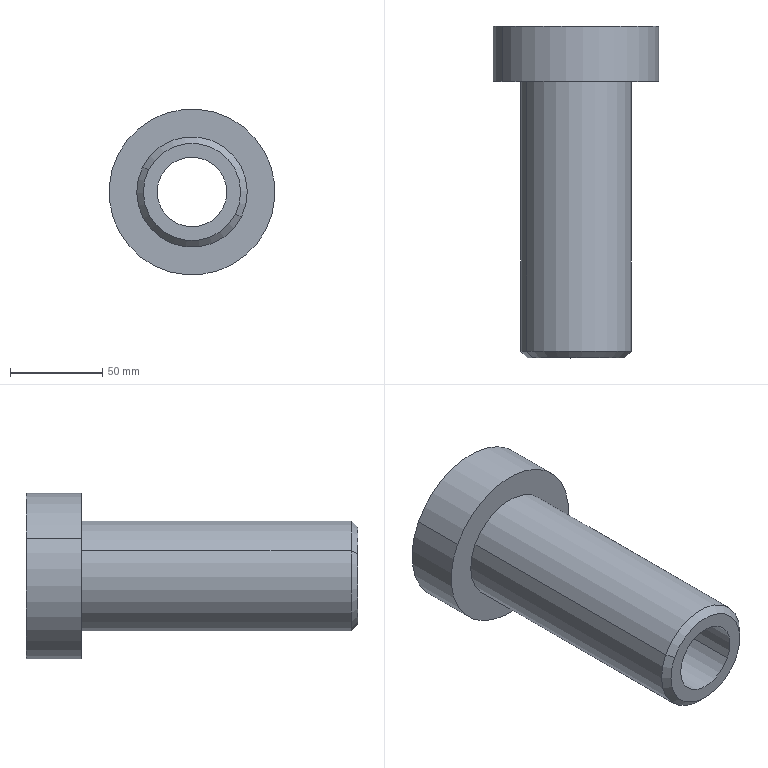Part | STEP file | Scale factor 1[11] | 1 solid | 11 faces | box 90 x 180 x 90 mm | volume 411797 mm3 | cylinder 6 | plane 3 | cone 2 | commonest cylinder face diameters 37.8 x2 60 x2 90 x2
STEP:
#1=CARTESIAN_POINT('',(-772.257,-401.273,3250.492));
#2=VERTEX_POINT('',#1);
#3=CARTESIAN_POINT('',(-725.219,-401.273,3226.508));
#4=VERTEX_POINT('',#3);
#5=CARTESIAN_POINT('',(-748.738,-401.273,3238.5));
#6=DIRECTION('',(0.,-1.,0.));
#7=DIRECTION('',(-0.8909,0.,0.4543));
#8=AXIS2_PLACEMENT_3D('',#5,#6,#7);
#9=CIRCLE('',#8,26.4);
#10=EDGE_CURVE('',#2,#4,#9,.T.);
#11=ORIENTED_EDGE('',*,*,#10,.F.);
#12=CARTESIAN_POINT('',(-775.464,-397.673,3252.128));
#13=VERTEX_POINT('',#12);
#14=CARTESIAN_POINT('',(-772.257,-401.273,3250.492));
#15=DIRECTION('',(-0.6299,0.7071,0.3212));
#16=VECTOR('',#15,1000.);
#17=LINE('',#14,#16);
#18=EDGE_CURVE('',#2,#13,#17,.T.);
#19=ORIENTED_EDGE('',*,*,#18,.T.);
#20=CARTESIAN_POINT('',(-722.012,-397.673,3224.872));
#21=VERTEX_POINT('',#20);
#22=CARTESIAN_POINT('',(-748.738,-397.673,3238.5));
#23=DIRECTION('',(0.,1.,0.));
#24=DIRECTION('',(-0.8909,0.,0.4543));
#25=AXIS2_PLACEMENT_3D('',#22,#23,#24);
#26=CIRCLE('',#25,30.);
#27=EDGE_CURVE('',#21,#13,#26,.T.);
#28=ORIENTED_EDGE('',*,*,#27,.F.);
#29=CARTESIAN_POINT('',(-725.219,-401.273,3226.508));
#30=DIRECTION('',(0.6299,0.7071,-0.3212));
#31=VECTOR('',#30,1000.);
#32=LINE('',#29,#31);
#33=EDGE_CURVE('',#4,#21,#32,.T.);
#34=ORIENTED_EDGE('',*,*,#33,.F.);
#35=EDGE_LOOP('',(#11,#19,#28,#34));
#36=FACE_OUTER_BOUND('',#35,.T.);
#37=CARTESIAN_POINT('',(-748.738,-401.273,3238.5));
#38=DIRECTION('',(0.,1.,0.));
#39=DIRECTION('',(-0.8909,0.,0.4543));
#40=AXIS2_PLACEMENT_3D('',#37,#38,#39);
#41=CONICAL_SURFACE('',#40,26.4,0.7854);
#42=ADVANCED_FACE('',(#36),#41,.T.);
#43=CARTESIAN_POINT('',(-731.901,-401.273,3229.915));
#44=VERTEX_POINT('',#43);
#45=CARTESIAN_POINT('',(-765.576,-401.273,3247.085));
#46=VERTEX_POINT('',#45);
#47=CARTESIAN_POINT('',(-748.738,-401.273,3238.5));
#48=DIRECTION('',(0.,-1.,0.));
#49=DIRECTION('',(-0.8909,0.,0.4543));
#50=AXIS2_PLACEMENT_3D('',#47,#48,#49);
#51=CIRCLE('',#50,18.9);
#52=EDGE_CURVE('',#44,#46,#51,.T.);
#53=ORIENTED_EDGE('',*,*,#52,.T.);
#54=CARTESIAN_POINT('',(-765.576,-221.273,3247.085));
#55=VERTEX_POINT('',#54);
#56=CARTESIAN_POINT('',(-765.576,-431.273,3247.085));
#57=DIRECTION('',(0.,1.,0.));
#58=VECTOR('',#57,1000.);
#59=LINE('',#56,#58);
#60=EDGE_CURVE('',#46,#55,#59,.T.);
#61=ORIENTED_EDGE('',*,*,#60,.T.);
#62=CARTESIAN_POINT('',(-731.901,-221.273,3229.915));
#63=VERTEX_POINT('',#62);
#64=CARTESIAN_POINT('',(-748.738,-221.273,3238.5));
#65=DIRECTION('',(0.,1.,0.));
#66=DIRECTION('',(0.8909,0.,-0.4543));
#67=AXIS2_PLACEMENT_3D('',#64,#65,#66);
#68=CIRCLE('',#67,18.9);
#69=EDGE_CURVE('',#55,#63,#68,.T.);
#70=ORIENTED_EDGE('',*,*,#69,.T.);
#71=CARTESIAN_POINT('',(-731.901,-431.273,3229.915));
#72=DIRECTION('',(0.,1.,0.));
#73=VECTOR('',#72,1000.);
#74=LINE('',#71,#73);
#75=EDGE_CURVE('',#44,#63,#74,.T.);
#76=ORIENTED_EDGE('',*,*,#75,.F.);
#77=EDGE_LOOP('',(#53,#61,#70,#76));
#78=FACE_OUTER_BOUND('',#77,.T.);
#79=CARTESIAN_POINT('',(-748.738,-431.273,3238.5));
#80=DIRECTION('',(0.,1.,0.));
#81=DIRECTION('',(-0.8909,0.,0.4543));
#82=AXIS2_PLACEMENT_3D('',#79,#80,#81);
#83=CYLINDRICAL_SURFACE('',#82,18.9);
#84=ADVANCED_FACE('',(#78),#83,.F.);
#85=ORIENTED_EDGE('',*,*,#27,.T.);
#86=CARTESIAN_POINT('',(-775.464,-251.273,3252.128));
#87=VERTEX_POINT('',#86);
#88=CARTESIAN_POINT('',(-775.464,-401.273,3252.128));
#89=DIRECTION('',(0.,1.,0.));
#90=VECTOR('',#89,1000.);
#91=LINE('',#88,#90);
#92=EDGE_CURVE('',#13,#87,#91,.T.);
#93=ORIENTED_EDGE('',*,*,#92,.T.);
#94=CARTESIAN_POINT('',(-722.012,-251.273,3224.872));
#95=VERTEX_POINT('',#94);
#96=CARTESIAN_POINT('',(-748.738,-251.273,3238.5));
#97=DIRECTION('',(0.,-1.,0.));
#98=DIRECTION('',(-0.8909,0.,0.4543));
#99=AXIS2_PLACEMENT_3D('',#96,#97,#98);
#100=CIRCLE('',#99,30.);
#101=EDGE_CURVE('',#87,#95,#100,.T.);
#102=ORIENTED_EDGE('',*,*,#101,.T.);
#103=CARTESIAN_POINT('',(-722.012,-401.273,3224.872));
#104=DIRECTION('',(0.,1.,0.));
#105=VECTOR('',#104,1000.);
#106=LINE('',#103,#105);
#107=EDGE_CURVE('',#21,#95,#106,.T.);
#108=ORIENTED_EDGE('',*,*,#107,.F.);
#109=EDGE_LOOP('',(#85,#93,#102,#108));
#110=FACE_OUTER_BOUND('',#109,.T.);
#111=CARTESIAN_POINT('',(-748.738,-401.273,3238.5));
#112=DIRECTION('',(0.,1.,0.));
#113=DIRECTION('',(-0.8909,0.,0.4543));
#114=AXIS2_PLACEMENT_3D('',#111,#112,#113);
#115=CYLINDRICAL_SURFACE('',#114,30.);
#116=ADVANCED_FACE('',(#110),#115,.T.);
#117=CARTESIAN_POINT('',(-788.827,-251.273,3258.942));
#118=VERTEX_POINT('',#117);
#119=CARTESIAN_POINT('',(-708.649,-251.273,3218.058));
#120=VERTEX_POINT('',#119);
#121=CARTESIAN_POINT('',(-748.738,-251.273,3238.5));
#122=DIRECTION('',(0.,-1.,0.));
#123=DIRECTION('',(-0.8909,0.,0.4543));
#124=AXIS2_PLACEMENT_3D('',#121,#122,#123);
#125=CIRCLE('',#124,45.);
#126=EDGE_CURVE('',#118,#120,#125,.T.);
#127=ORIENTED_EDGE('',*,*,#126,.F.);
#128=CARTESIAN_POINT('',(-788.827,-221.273,3258.942));
#129=VERTEX_POINT('',#128);
#130=CARTESIAN_POINT('',(-788.827,-251.273,3258.942));
#131=DIRECTION('',(0.,1.,0.));
#132=VECTOR('',#131,1000.);
#133=LINE('',#130,#132);
#134=EDGE_CURVE('',#118,#129,#133,.T.);
#135=ORIENTED_EDGE('',*,*,#134,.T.);
#136=CARTESIAN_POINT('',(-708.649,-221.273,3218.058));
#137=VERTEX_POINT('',#136);
#138=CARTESIAN_POINT('',(-748.738,-221.273,3238.5));
#139=DIRECTION('',(0.,-1.,0.));
#140=DIRECTION('',(-0.8909,0.,0.4543));
#141=AXIS2_PLACEMENT_3D('',#138,#139,#140);
#142=CIRCLE('',#141,45.);
#143=EDGE_CURVE('',#129,#137,#142,.T.);
#144=ORIENTED_EDGE('',*,*,#143,.T.);
#145=CARTESIAN_POINT('',(-708.649,-251.273,3218.058));
#146=DIRECTION('',(0.,1.,0.));
#147=VECTOR('',#146,1000.);
#148=LINE('',#145,#147);
#149=EDGE_CURVE('',#120,#137,#148,.T.);
#150=ORIENTED_EDGE('',*,*,#149,.F.);
#151=EDGE_LOOP('',(#127,#135,#144,#150));
#152=FACE_OUTER_BOUND('',#151,.T.);
#153=CARTESIAN_POINT('',(-748.738,-251.273,3238.5));
#154=DIRECTION('',(0.,1.,0.));
#155=DIRECTION('',(-0.8909,0.,0.4543));
#156=AXIS2_PLACEMENT_3D('',#153,#154,#155);
#157=CYLINDRICAL_SURFACE('',#156,45.);
#158=ADVANCED_FACE('',(#152),#157,.T.);
#159=ORIENTED_EDGE('',*,*,#134,.F.);
#160=CARTESIAN_POINT('',(-748.738,-251.273,3238.5));
#161=DIRECTION('',(0.,-1.,0.));
#162=DIRECTION('',(-0.8909,0.,0.4543));
#163=AXIS2_PLACEMENT_3D('',#160,#161,#162);
#164=CIRCLE('',#163,45.);
#165=EDGE_CURVE('',#120,#118,#164,.T.);
#166=ORIENTED_EDGE('',*,*,#165,.F.);
#167=ORIENTED_EDGE('',*,*,#149,.T.);
#168=CARTESIAN_POINT('',(-748.738,-221.273,3238.5));
#169=DIRECTION('',(0.,-1.,0.));
#170=DIRECTION('',(-0.8909,0.,0.4543));
#171=AXIS2_PLACEMENT_3D('',#168,#169,#170);
#172=CIRCLE('',#171,45.);
#173=EDGE_CURVE('',#137,#129,#172,.T.);
#174=ORIENTED_EDGE('',*,*,#173,.T.);
#175=EDGE_LOOP('',(#159,#166,#167,#174));
#176=FACE_OUTER_BOUND('',#175,.T.);
#177=CARTESIAN_POINT('',(-748.738,-251.273,3238.5));
#178=DIRECTION('',(0.,1.,0.));
#179=DIRECTION('',(-0.8909,0.,0.4543));
#180=AXIS2_PLACEMENT_3D('',#177,#178,#179);
#181=CYLINDRICAL_SURFACE('',#180,45.);
#182=ADVANCED_FACE('',(#176),#181,.T.);
#183=CARTESIAN_POINT('',(-748.738,-251.273,3238.5));
#184=DIRECTION('',(0.,-1.,0.));
#185=DIRECTION('',(-0.8909,0.,0.4543));
#186=AXIS2_PLACEMENT_3D('',#183,#184,#185);
#187=CIRCLE('',#186,30.);
#188=EDGE_CURVE('',#95,#87,#187,.T.);
#189=ORIENTED_EDGE('',*,*,#188,.F.);
#190=ORIENTED_EDGE('',*,*,#101,.F.);
#191=EDGE_LOOP('',(#189,#190));
#192=FACE_BOUND('',#191,.T.);
#193=ORIENTED_EDGE('',*,*,#165,.T.);
#194=ORIENTED_EDGE('',*,*,#126,.T.);
#195=EDGE_LOOP('',(#193,#194));
#196=FACE_OUTER_BOUND('',#195,.T.);
#197=CARTESIAN_POINT('',(-748.738,-251.273,3238.5));
#198=DIRECTION('',(0.,-1.,0.));
#199=DIRECTION('',(0.8909,0.,-0.4543));
#200=AXIS2_PLACEMENT_3D('',#197,#198,#199);
#201=PLANE('',#200);
#202=ADVANCED_FACE('',(#192,#196),#201,.T.);
#203=CARTESIAN_POINT('',(-748.738,-221.273,3238.5));
#204=DIRECTION('',(0.,1.,0.));
#205=DIRECTION('',(0.8909,0.,-0.4543));
#206=AXIS2_PLACEMENT_3D('',#203,#204,#205);
#207=CIRCLE('',#206,18.9);
#208=EDGE_CURVE('',#63,#55,#207,.T.);
#209=ORIENTED_EDGE('',*,*,#208,.F.);
#210=ORIENTED_EDGE('',*,*,#69,.F.);
#211=EDGE_LOOP('',(#209,#210));
#212=FACE_BOUND('',#211,.T.);
#213=ORIENTED_EDGE('',*,*,#173,.F.);
#214=ORIENTED_EDGE('',*,*,#143,.F.);
#215=EDGE_LOOP('',(#213,#214));
#216=FACE_OUTER_BOUND('',#215,.T.);
#217=CARTESIAN_POINT('',(-748.738,-221.273,3238.5));
#218=DIRECTION('',(0.,-1.,0.));
#219=DIRECTION('',(0.8909,0.,-0.4543));
#220=AXIS2_PLACEMENT_3D('',#217,#218,#219);
#221=PLANE('',#220);
#222=ADVANCED_FACE('',(#212,#216),#221,.F.);
#223=ORIENTED_EDGE('',*,*,#92,.F.);
#224=CARTESIAN_POINT('',(-748.738,-397.673,3238.5));
#225=DIRECTION('',(0.,1.,0.));
#226=DIRECTION('',(-0.8909,0.,0.4543));
#227=AXIS2_PLACEMENT_3D('',#224,#225,#226);
#228=CIRCLE('',#227,30.);
#229=EDGE_CURVE('',#13,#21,#228,.T.);
#230=ORIENTED_EDGE('',*,*,#229,.T.);
#231=ORIENTED_EDGE('',*,*,#107,.T.);
#232=ORIENTED_EDGE('',*,*,#188,.T.);
#233=EDGE_LOOP('',(#223,#230,#231,#232));
#234=FACE_OUTER_BOUND('',#233,.T.);
#235=CARTESIAN_POINT('',(-748.738,-401.273,3238.5));
#236=DIRECTION('',(0.,1.,0.));
#237=DIRECTION('',(-0.8909,0.,0.4543));
#238=AXIS2_PLACEMENT_3D('',#235,#236,#237);
#239=CYLINDRICAL_SURFACE('',#238,30.);
#240=ADVANCED_FACE('',(#234),#239,.T.);
#241=CARTESIAN_POINT('',(-748.738,-401.273,3238.5));
#242=DIRECTION('',(0.,-1.,0.));
#243=DIRECTION('',(-0.8909,0.,0.4543));
#244=AXIS2_PLACEMENT_3D('',#241,#242,#243);
#245=CIRCLE('',#244,26.4);
#246=EDGE_CURVE('',#4,#2,#245,.T.);
#247=ORIENTED_EDGE('',*,*,#246,.T.);
#248=ORIENTED_EDGE('',*,*,#10,.T.);
#249=EDGE_LOOP('',(#247,#248));
#250=FACE_OUTER_BOUND('',#249,.T.);
#251=ORIENTED_EDGE('',*,*,#52,.F.);
#252=CARTESIAN_POINT('',(-748.738,-401.273,3238.5));
#253=DIRECTION('',(0.,-1.,0.));
#254=DIRECTION('',(-0.8909,0.,0.4543));
#255=AXIS2_PLACEMENT_3D('',#252,#253,#254);
#256=CIRCLE('',#255,18.9);
#257=EDGE_CURVE('',#46,#44,#256,.T.);
#258=ORIENTED_EDGE('',*,*,#257,.F.);
#259=EDGE_LOOP('',(#251,#258));
#260=FACE_BOUND('',#259,.T.);
#261=CARTESIAN_POINT('',(-748.738,-401.273,3238.5));
#262=DIRECTION('',(0.,-1.,0.));
#263=DIRECTION('',(0.8909,0.,-0.4543));
#264=AXIS2_PLACEMENT_3D('',#261,#262,#263);
#265=PLANE('',#264);
#266=ADVANCED_FACE('',(#250,#260),#265,.T.);
#267=ORIENTED_EDGE('',*,*,#60,.F.);
#268=ORIENTED_EDGE('',*,*,#257,.T.);
#269=ORIENTED_EDGE('',*,*,#75,.T.);
#270=ORIENTED_EDGE('',*,*,#208,.T.);
#271=EDGE_LOOP('',(#267,#268,#269,#270));
#272=FACE_OUTER_BOUND('',#271,.T.);
#273=CARTESIAN_POINT('',(-748.738,-431.273,3238.5));
#274=DIRECTION('',(0.,1.,0.));
#275=DIRECTION('',(-0.8909,0.,0.4543));
#276=AXIS2_PLACEMENT_3D('',#273,#274,#275);
#277=CYLINDRICAL_SURFACE('',#276,18.9);
#278=ADVANCED_FACE('',(#272),#277,.F.);
#279=ORIENTED_EDGE('',*,*,#18,.F.);
#280=ORIENTED_EDGE('',*,*,#246,.F.);
#281=ORIENTED_EDGE('',*,*,#33,.T.);
#282=ORIENTED_EDGE('',*,*,#229,.F.);
#283=EDGE_LOOP('',(#279,#280,#281,#282));
#284=FACE_OUTER_BOUND('',#283,.T.);
#285=CARTESIAN_POINT('',(-748.738,-401.273,3238.5));
#286=DIRECTION('',(0.,1.,0.));
#287=DIRECTION('',(-0.8909,0.,0.4543));
#288=AXIS2_PLACEMENT_3D('',#285,#286,#287);
#289=CONICAL_SURFACE('',#288,26.4,0.7854);
#290=ADVANCED_FACE('',(#284),#289,.T.);
#291=CLOSED_SHELL('',(#42,#84,#116,#158,#182,#202,#222,#240,#266,#278,#290));
#292=MANIFOLD_SOLID_BREP('',#291);
#293=CARTESIAN_POINT('',(0.,0.,0.));
#294=DIRECTION('',(0.,0.,1.));
#295=DIRECTION('',(1.,0.,0.));
#296=AXIS2_PLACEMENT_3D('',#293,#294,#295);
#297=(LENGTH_UNIT()NAMED_UNIT(*)SI_UNIT(.MILLI.,.METRE.));
#298=UNCERTAINTY_MEASURE_WITH_UNIT(LENGTH_MEASURE(0.00001),#297,'','');
#299=(NAMED_UNIT(*)PLANE_ANGLE_UNIT()SI_UNIT($,.RADIAN.));
#300=(NAMED_UNIT(*)SI_UNIT($,.STERADIAN.)SOLID_ANGLE_UNIT());
#301=(GEOMETRIC_REPRESENTATION_CONTEXT(3)GLOBAL_UNCERTAINTY_ASSIGNED_CONTEXT((#298))GLOBAL_UNIT_ASSIGNED_CONTEXT((#297,#299,#300))REPRESENTATION_CONTEXT('',''));
#302=ADVANCED_BREP_SHAPE_REPRESENTATION('',(#292,#296),#301);